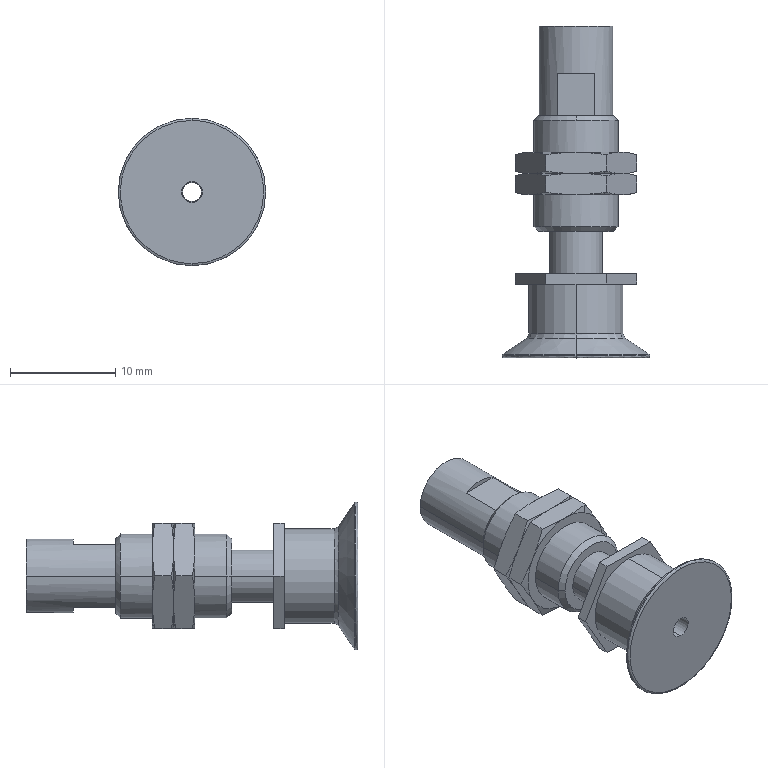Part | SolidWorks | features BaseBody 4 | 4 solids | 103 faces | box 14 x 31.5 x 14 mm | volume 1615 mm3 | cone 46 | plane 33 | cylinder 20 | spline 4 | commonest cylinder face diameters 7.188 x4 1.8 x2 2 x2 4.134 x2 5 x2 7 x2